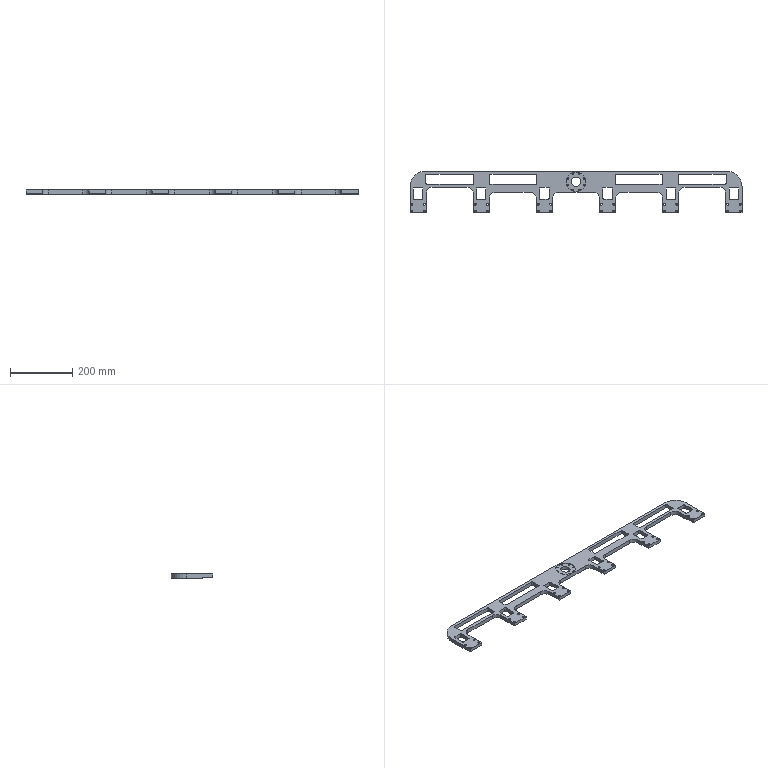NC program | NX | posted with a generic post | part box 1068 x 134 x 13 mm
Lines 3824 to 4175 of 4175:
(PLANAR_MILL_COPY_1_COPY , TOOL : D6A45)
N7598 T07 M6
N7600 G54
N7602 G17 G0 G90 X520.9 Y-5.27 S9500 M3
N7604 G43 Z30. H7
N7606 Z0.
N7608 G94 G1 Z-1. F1400.
N7610 X521.6 Y-4.866
N7612 G3 X522.1 Y-4. R1.
N7614 G1 Y13.
N7616 G3 X520. Y15.1 R2.1
N7618 G1 X496.
N7620 G3 X493.9 Y13. R2.1
N7622 G1 Y-21.
N7624 G3 X496. Y-23.1 R2.1
N7626 G1 X520.
N7628 G3 X522.1 Y-21. R2.1
N7630 G1 Y-4.
N7632 G3 X521.6 Y-3.134 R1.
N7634 G1 X520.9 Y-2.73
N7636 Z0.
N7638 G0 Z30.
N7640 X407.67 Y54.9
N7642 Z0.
N7644 G1 Z-1.
N7646 X407.266 Y55.6
N7648 G3 X406.4 Y56.1 R1.
N7650 G1 X332.8
N7652 G3 X330.7 Y54. R2.1
N7654 G1 Y28.
N7656 G3 X332.8 Y25.9 R2.1
N7658 G1 X480.
N7660 G3 X482.1 Y28. R2.1
N7662 G1 Y54.
N7664 G3 X480. Y56.1 R2.1
N7666 G1 X406.4
N7668 G3 X405.534 Y55.6 R1.
N7670 G1 X405.13 Y54.9
N7672 Z0.
N7674 G0 Z30.
N7676 X116.33 Y69.1
N7678 Z0.
N7680 G1 Z-1.
N7682 X116.734 Y68.4
N7684 G3 X117.6 Y67.9 R1.
N7686 G1 X484.
N7688 G2 X534.9 Y17. R50.9
N7690 G1 Y-33.3
N7692 G2 X533.9 Y-34.3 R1.
N7694 G1 X482.1
N7696 G2 X481.1 Y-33.3 R1.
N7698 G1 Y-5.
N7700 G3 X462. Y14.1 R19.1
N7702 G1 X350.8
N7704 G3 X331.7 Y-5. R19.1
N7706 G1 Y-33.3
N7708 G2 X330.7 Y-34.3 R1.
N7710 G1 X278.9
N7712 G2 X277.9 Y-33.3 R1.
N7714 G1 Y-20.95
N7716 G3 X258.8 Y-1.85 R19.1
N7718 G1 X147.6
N7720 G3 X128.5 Y-20.95 R19.1
N7722 G1 Y-33.3
N7724 G2 X127.5 Y-34.3 R1.
N7726 G1 X117.6
N7728 G3 X116.734 Y-34.8 R1.
N7730 G1 X116.33 Y-35.5
N7732 Z0.
N7734 G0 Z30.
N7736 X291.9 Y-2.73
N7738 Z0.
N7740 G1 Z-1.
N7742 X291.2 Y-3.134
N7744 G3 X290.7 Y-4. R1.
N7746 G1 Y-21.
N7748 G3 X292.8 Y-23.1 R2.1
N7750 G1 X316.8
N7752 G3 X318.9 Y-21. R2.1
N7754 G1 Y13.
N7756 G3 X316.8 Y15.1 R2.1
N7758 G1 X292.8
N7760 G3 X290.7 Y13. R2.1
N7762 G1 Y-4.
N7764 G3 X291.2 Y-4.866 R1.
N7766 G1 X291.9 Y-5.27
N7768 Z0.
N7770 G0 Z30.
N7772 X204.47 Y54.9
N7774 Z0.
N7776 G1 Z-1.
N7778 X204.066 Y55.6
N7780 G3 X203.2 Y56.1 R1.
N7782 G1 X129.6
N7784 G3 X127.5 Y54. R2.1
N7786 G1 Y28.
N7788 G3 X129.6 Y25.9 R2.1
N7790 G1 X276.8
N7792 G3 X278.9 Y28. R2.1
N7794 G1 Y54.
N7796 G3 X276.8 Y56.1 R2.1
N7798 G1 X203.2
N7800 G3 X202.334 Y55.6 R1.
N7802 G1 X201.93 Y54.9
N7804 Z0.
N7806 G0 Z30.
(PLANAR_MILL_COPY_COPY_COPY , TOOL : D6A45)
N7808 X527.993 Y-38.1
N7810 Z-3.
N7812 G1 Z-4.
N7814 Y-37.056
N7816 G3 X527.518 Y-36.9 R0.5
N7818 X528.482 Y-36.9 R-2.35
N7820 X528.007 Y-37.056 R0.5
N7822 G1 Y-38.1
N7824 Z-3.
N7826 G0 Z30.
N7828 X527.512 Y-62.242
N7830 Z-3.
N7832 G1 Z-4.
N7834 X527.134 Y-63.05
N7836 G3 X528. Y-63.55 R1.
N7838 X530.35 Y-61.2 R2.35
N7840 X528. Y-63.55 R-2.35
N7842 X528.866 Y-63.05 R1.
N7844 G1 X528.488 Y-62.242
N7846 Z-3.
N7848 G0 Z30.
N7850 X487.512
N7852 Z-3.
N7854 G1 Z-4.
N7856 X487.134 Y-63.05
N7858 G3 X488. Y-63.55 R1.
N7860 X490.35 Y-61.2 R2.35
N7862 X488. Y-63.55 R-2.35
N7864 X488.866 Y-63.05 R1.
N7866 G1 X488.488 Y-62.242
N7868 Z-3.
N7870 G0 Z30.
N7872 X487.993 Y-38.1
N7874 Z-3.
N7876 G1 Z-4.
N7878 Y-37.056
N7880 G3 X487.518 Y-36.9 R0.5
N7882 X488.482 Y-36.9 R-2.35
N7884 X488.007 Y-37.056 R0.5
N7886 G1 Y-38.1
N7888 Z-3.
N7890 G0 Z30.
N7892 X536.313 Y-37.492
N7894 Z-3.
N7896 G1 Z-4.
N7898 X535.865 Y-37.043
N7900 G3 X534.9 Y-36.782 R1.
N7902 G1 Y-66.9
N7904 G2 X533.9 Y-67.9 R1.
N7906 G1 X482.1
N7908 G2 X481.1 Y-66.9 R1.
N7910 G1 Y-36.782
N7912 G3 X480.135 Y-37.043 R1.
N7914 G1 X479.687 Y-37.492
N7916 Z-3.
N7918 G0 Z30.
N7920 X333.113
N7922 Z-3.
N7924 G1 Z-4.
N7926 X332.665 Y-37.043
N7928 G3 X331.7 Y-36.782 R1.
N7930 G1 Y-66.9
N7932 G2 X330.7 Y-67.9 R1.
N7934 G1 X278.9
N7936 G2 X277.9 Y-66.9 R1.
N7938 G1 Y-36.782
N7940 G3 X276.935 Y-37.043 R1.
N7942 G1 X276.487 Y-37.492
N7944 Z-3.
N7946 G0 Z30.
N7948 X324.793 Y-38.1
N7950 Z-3.
N7952 G1 Z-4.
N7954 Y-37.056
N7956 G3 X324.318 Y-36.9 R0.5
N7958 X325.282 Y-36.9 R-2.35
N7960 X324.807 Y-37.056 R0.5
N7962 G1 Y-38.1
N7964 Z-3.
N7966 G0 Z30.
N7968 X324.312 Y-62.242
N7970 Z-3.
N7972 G1 Z-4.
N7974 X323.934 Y-63.05
N7976 G3 X324.8 Y-63.55 R1.
N7978 X327.15 Y-61.2 R2.35
N7980 X324.8 Y-63.55 R-2.35
N7982 X325.666 Y-63.05 R1.
N7984 G1 X325.288 Y-62.242
N7986 Z-3.
N7988 G0 Z30.
N7990 X284.312
N7992 Z-3.
N7994 G1 Z-4.
N7996 X283.934 Y-63.05
N7998 G3 X284.8 Y-63.55 R1.
N8000 X287.15 Y-61.2 R2.35
N8002 X284.8 Y-63.55 R-2.35
N8004 X285.666 Y-63.05 R1.
N8006 G1 X285.288 Y-62.242
N8008 Z-3.
N8010 G0 Z30.
N8012 X284.793 Y-38.1
N8014 Z-3.
N8016 G1 Z-4.
N8018 Y-37.056
N8020 G3 X284.318 Y-36.9 R0.5
N8022 X285.282 Y-36.9 R-2.35
N8024 X284.807 Y-37.056 R0.5
N8026 G1 Y-38.1
N8028 Z-3.
N8030 G0 Z30.
N8032 M5
(ZLEVEL_PROFILE_COPY_3_COPY_COPY , TOOL : D10)
N8034 T10 M6
N8036 G54
N8038 G17 G0 G90 X115.002 Y75.5 S9500 M3
N8040 G43 Z30. H10
N8042 Z-7.525
N8044 G94 G1 Z-12.525 F1000.
N8046 X116.734 Y72.5
N8048 G3 X117.6 Y72. R1.
N8050 G1 X484. F1200.
N8052 G2 X539. Y17. R55.
N8054 G1 Y-67.
N8056 G2 X534. Y-72. R5.
N8058 G1 X482.
N8060 G2 X477. Y-67. R5.
N8062 G1 Y-5.
N8064 G3 X462. Y10. R15.
N8066 G1 X350.8
N8068 G3 X335.8 Y-5. R15.
N8070 G1 Y-67.
N8072 G2 X330.8 Y-72. R5.
N8074 G1 X278.8
N8076 G2 X273.8 Y-67. R5.
N8078 G1 Y-20.95
N8080 G3 X258.8 Y-5.95 R15.
N8082 G1 X147.6
N8084 G3 X132.6 Y-20.95 R15.
N8086 G1 Y-67.
N8088 G2 X127.6 Y-72. R5.
N8090 G1 X117.6
N8092 G3 X116.734 Y-72.5 R1.
N8094 G1 X115.002 Y-75.5
N8096 Z-7.525
N8098 G0 Z30.
N8100 Y75.5
N8102 Z-7.65
N8104 G1 Z-12.65 F1000.
N8106 X116.734 Y72.5
N8108 G3 X117.6 Y72. R1.
N8110 G1 X484. F1200.
N8112 G2 X539. Y17. R55.
N8114 G1 Y-67.
N8116 G2 X534. Y-72. R5.
N8118 G1 X482.
N8120 G2 X477. Y-67. R5.
N8122 G1 Y-5.
N8124 G3 X462. Y10. R15.
N8126 G1 X350.8
N8128 G3 X335.8 Y-5. R15.
N8130 G1 Y-67.
N8132 G2 X330.8 Y-72. R5.
N8134 G1 X278.8
N8136 G2 X273.8 Y-67. R5.
N8138 G1 Y-20.95
N8140 G3 X258.8 Y-5.95 R15.
N8142 G1 X147.6
N8144 G3 X132.6 Y-20.95 R15.
N8146 G1 Y-67.
N8148 G2 X127.6 Y-72. R5.
N8150 G1 X117.6
N8152 G3 X116.734 Y-72.5 R1.
N8154 G1 X115.002 Y-75.5
N8156 Z-7.65
N8158 G0 Z30.
N8160 Y75.5
N8162 Z-7.775
N8164 G1 Z-12.775 F1000.
N8166 X116.734 Y72.5
N8168 G3 X117.6 Y72. R1.
N8170 G1 X484. F1200.
N8172 G2 X539. Y17. R55.
N8174 G1 Y-67.
N8176 G2 X534. Y-72. R5.
N8178 G1 X482.
N8180 G2 X477. Y-67. R5.
N8182 G1 Y-5.
N8184 G3 X462. Y10. R15.
N8186 G1 X350.8
N8188 G3 X335.8 Y-5. R15.
N8190 G1 Y-67.
N8192 G2 X330.8 Y-72. R5.
N8194 G1 X278.8
N8196 G2 X273.8 Y-67. R5.
N8198 G1 Y-20.95
N8200 G3 X258.8 Y-5.95 R15.
N8202 G1 X147.6
N8204 G3 X132.6 Y-20.95 R15.
N8206 G1 Y-67.
N8208 G2 X127.6 Y-72. R5.
N8210 G1 X117.6
N8212 G3 X116.734 Y-72.5 R1.
N8214 G1 X115.002 Y-75.5
N8216 Z-7.775
N8218 G0 Z30.
N8220 Y75.5
N8222 Z-7.9
N8224 G1 Z-12.9 F1000.
N8226 X116.734 Y72.5
N8228 G3 X117.6 Y72. R1.
N8230 G1 X484. F1200.
N8232 G2 X539. Y17. R55.
N8234 G1 Y-67.
N8236 G2 X534. Y-72. R5.
N8238 G1 X482.
N8240 G2 X477. Y-67. R5.
N8242 G1 Y-5.
N8244 G3 X462. Y10. R15.
N8246 G1 X350.8
N8248 G3 X335.8 Y-5. R15.
N8250 G1 Y-67.
N8252 G2 X330.8 Y-72. R5.
N8254 G1 X278.8
N8256 G2 X273.8 Y-67. R5.
N8258 G1 Y-20.95
N8260 G3 X258.8 Y-5.95 R15.
N8262 G1 X147.6
N8264 G3 X132.6 Y-20.95 R15.
N8266 G1 Y-67.
N8268 G2 X127.6 Y-72. R5.
N8270 G1 X117.6
N8272 G3 X116.734 Y-72.5 R1.
N8274 G1 X115.002 Y-75.5
N8276 Z-7.9
N8278 G0 Z30.
N8280 M5
N8282 M2